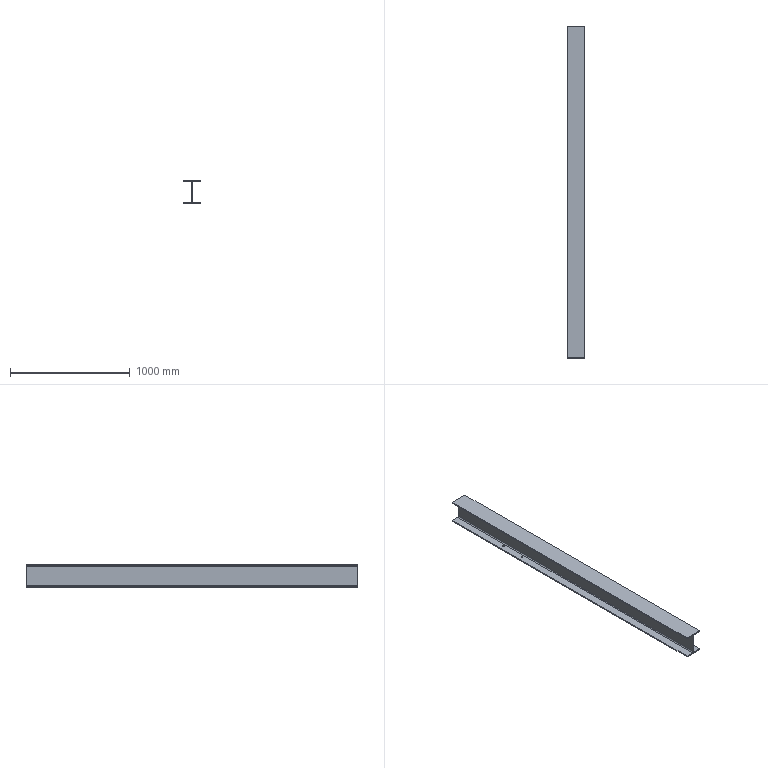Part | STEP file | 计量立柱1主体_Default<As Machined> | 1 solid | 26 faces | box 150 x 2778 x 194 mm | volume 10580424 mm3 | plane 14 | cylinder 12 | commonest cylinder face diameters 15 x8 16 x4